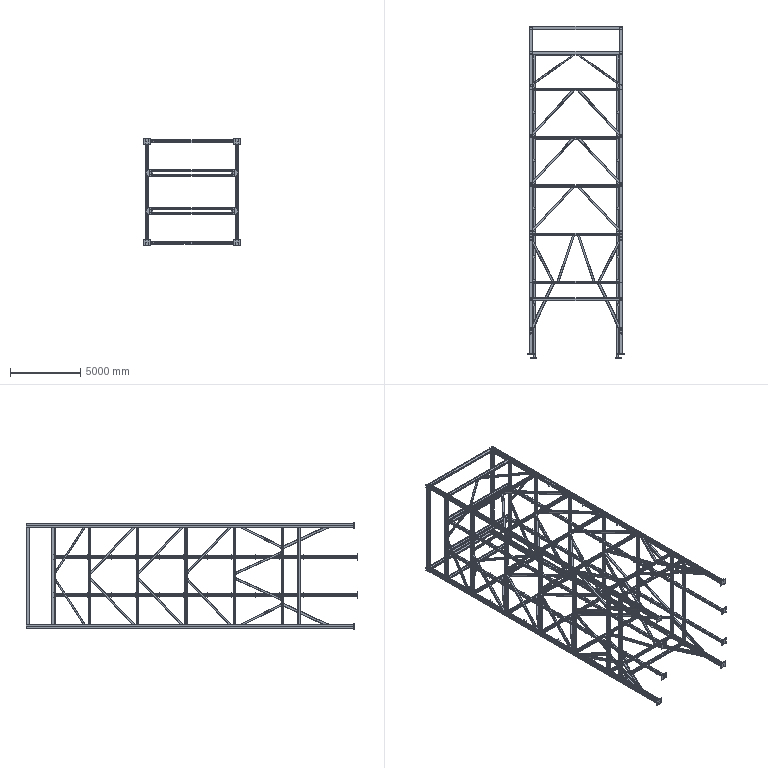Part | STEP file | Steel structure_default<machining> | 380 solids | 5328 faces | volume 3257360996 mm3 | plane 3768 | cylinder 1560 | commonest cylinder face diameters 18 x480 32 x368 6.66 x240 16 x192 24 x120 26 x48